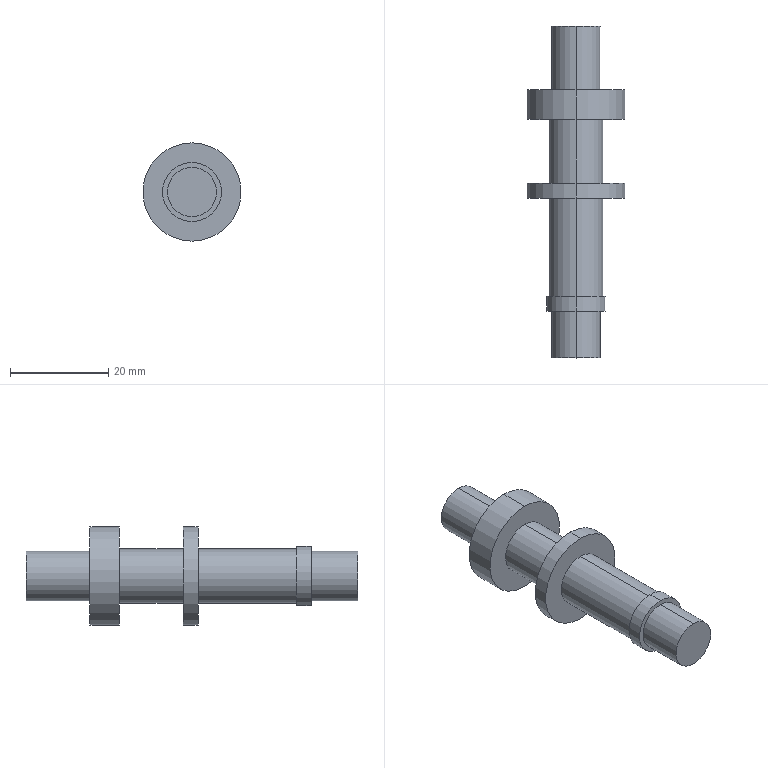Part | SolidWorks | features Revolution 1 | 1 solid | 22 faces | box 20 x 67.5 x 20 mm | volume 8070 mm3 | cylinder 14 | plane 8 | commonest cylinder face diameters 10 x4 11 x4 20 x4 12 x2
STEP:
#1=CARTESIAN_POINT('',(0.,67.5,-5.));
#2=VERTEX_POINT('',#1);
#3=CARTESIAN_POINT('',(0.,67.5,5.));
#4=VERTEX_POINT('',#3);
#5=CARTESIAN_POINT('',(0.,67.5,0.));
#6=DIRECTION('',(0.,-1.,0.));
#7=DIRECTION('',(0.,0.,-1.));
#8=AXIS2_PLACEMENT_3D('',#5,#6,#7);
#9=CIRCLE('',#8,5.);
#10=EDGE_CURVE('',#2,#4,#9,.T.);
#11=ORIENTED_EDGE('',*,*,#10,.T.);
#12=CARTESIAN_POINT('',(0.,54.5,5.));
#13=VERTEX_POINT('',#12);
#14=CARTESIAN_POINT('',(0.,-28.718,5.));
#15=DIRECTION('',(0.,-1.,0.));
#16=VECTOR('',#15,1000.);
#17=LINE('',#14,#16);
#18=EDGE_CURVE('',#4,#13,#17,.T.);
#19=ORIENTED_EDGE('',*,*,#18,.T.);
#20=CARTESIAN_POINT('',(0.,54.5,-5.));
#21=VERTEX_POINT('',#20);
#22=CARTESIAN_POINT('',(0.,54.5,0.));
#23=DIRECTION('',(0.,-1.,0.));
#24=DIRECTION('',(0.,0.,-1.));
#25=AXIS2_PLACEMENT_3D('',#22,#23,#24);
#26=CIRCLE('',#25,5.);
#27=EDGE_CURVE('',#21,#13,#26,.T.);
#28=ORIENTED_EDGE('',*,*,#27,.F.);
#29=CARTESIAN_POINT('',(0.,-28.718,-5.));
#30=DIRECTION('',(0.,-1.,0.));
#31=VECTOR('',#30,1000.);
#32=LINE('',#29,#31);
#33=EDGE_CURVE('',#2,#21,#32,.T.);
#34=ORIENTED_EDGE('',*,*,#33,.F.);
#35=EDGE_LOOP('',(#11,#19,#28,#34));
#36=FACE_OUTER_BOUND('',#35,.T.);
#37=CARTESIAN_POINT('',(0.,-28.718,0.));
#38=DIRECTION('',(0.,-1.,0.));
#39=DIRECTION('',(0.,0.,-1.));
#40=AXIS2_PLACEMENT_3D('',#37,#38,#39);
#41=CYLINDRICAL_SURFACE('',#40,5.);
#42=ADVANCED_FACE('',(#36),#41,.T.);
#43=CARTESIAN_POINT('',(0.,54.5,-10.));
#44=VERTEX_POINT('',#43);
#45=CARTESIAN_POINT('',(0.,54.5,10.));
#46=VERTEX_POINT('',#45);
#47=CARTESIAN_POINT('',(0.,54.5,0.));
#48=DIRECTION('',(0.,-1.,0.));
#49=DIRECTION('',(0.,0.,-1.));
#50=AXIS2_PLACEMENT_3D('',#47,#48,#49);
#51=CIRCLE('',#50,10.);
#52=EDGE_CURVE('',#44,#46,#51,.T.);
#53=ORIENTED_EDGE('',*,*,#52,.T.);
#54=CARTESIAN_POINT('',(0.,48.5,10.));
#55=VERTEX_POINT('',#54);
#56=CARTESIAN_POINT('',(0.,-28.718,10.));
#57=DIRECTION('',(0.,-1.,0.));
#58=VECTOR('',#57,1000.);
#59=LINE('',#56,#58);
#60=EDGE_CURVE('',#46,#55,#59,.T.);
#61=ORIENTED_EDGE('',*,*,#60,.T.);
#62=CARTESIAN_POINT('',(0.,48.5,-10.));
#63=VERTEX_POINT('',#62);
#64=CARTESIAN_POINT('',(0.,48.5,0.));
#65=DIRECTION('',(0.,-1.,0.));
#66=DIRECTION('',(0.,0.,-1.));
#67=AXIS2_PLACEMENT_3D('',#64,#65,#66);
#68=CIRCLE('',#67,10.);
#69=EDGE_CURVE('',#63,#55,#68,.T.);
#70=ORIENTED_EDGE('',*,*,#69,.F.);
#71=CARTESIAN_POINT('',(0.,-28.718,-10.));
#72=DIRECTION('',(0.,-1.,0.));
#73=VECTOR('',#72,1000.);
#74=LINE('',#71,#73);
#75=EDGE_CURVE('',#44,#63,#74,.T.);
#76=ORIENTED_EDGE('',*,*,#75,.F.);
#77=EDGE_LOOP('',(#53,#61,#70,#76));
#78=FACE_OUTER_BOUND('',#77,.T.);
#79=CARTESIAN_POINT('',(0.,-28.718,0.));
#80=DIRECTION('',(0.,-1.,0.));
#81=DIRECTION('',(0.,0.,-1.));
#82=AXIS2_PLACEMENT_3D('',#79,#80,#81);
#83=CYLINDRICAL_SURFACE('',#82,10.);
#84=ADVANCED_FACE('',(#78),#83,.T.);
#85=CARTESIAN_POINT('',(0.,48.5,-5.5));
#86=VERTEX_POINT('',#85);
#87=CARTESIAN_POINT('',(0.,48.5,5.5));
#88=VERTEX_POINT('',#87);
#89=CARTESIAN_POINT('',(0.,48.5,0.));
#90=DIRECTION('',(0.,-1.,0.));
#91=DIRECTION('',(0.,0.,-1.));
#92=AXIS2_PLACEMENT_3D('',#89,#90,#91);
#93=CIRCLE('',#92,5.5);
#94=EDGE_CURVE('',#86,#88,#93,.T.);
#95=ORIENTED_EDGE('',*,*,#94,.T.);
#96=CARTESIAN_POINT('',(0.,35.5,5.5));
#97=VERTEX_POINT('',#96);
#98=CARTESIAN_POINT('',(0.,-28.718,5.5));
#99=DIRECTION('',(0.,-1.,0.));
#100=VECTOR('',#99,1000.);
#101=LINE('',#98,#100);
#102=EDGE_CURVE('',#88,#97,#101,.T.);
#103=ORIENTED_EDGE('',*,*,#102,.T.);
#104=CARTESIAN_POINT('',(0.,35.5,-5.5));
#105=VERTEX_POINT('',#104);
#106=CARTESIAN_POINT('',(0.,35.5,0.));
#107=DIRECTION('',(0.,-1.,0.));
#108=DIRECTION('',(0.,0.,-1.));
#109=AXIS2_PLACEMENT_3D('',#106,#107,#108);
#110=CIRCLE('',#109,5.5);
#111=EDGE_CURVE('',#105,#97,#110,.T.);
#112=ORIENTED_EDGE('',*,*,#111,.F.);
#113=CARTESIAN_POINT('',(0.,-28.718,-5.5));
#114=DIRECTION('',(0.,-1.,0.));
#115=VECTOR('',#114,1000.);
#116=LINE('',#113,#115);
#117=EDGE_CURVE('',#86,#105,#116,.T.);
#118=ORIENTED_EDGE('',*,*,#117,.F.);
#119=EDGE_LOOP('',(#95,#103,#112,#118));
#120=FACE_OUTER_BOUND('',#119,.T.);
#121=CARTESIAN_POINT('',(0.,-28.718,0.));
#122=DIRECTION('',(0.,-1.,0.));
#123=DIRECTION('',(0.,0.,-1.));
#124=AXIS2_PLACEMENT_3D('',#121,#122,#123);
#125=CYLINDRICAL_SURFACE('',#124,5.5);
#126=ADVANCED_FACE('',(#120),#125,.T.);
#127=CARTESIAN_POINT('',(0.,35.5,-10.));
#128=VERTEX_POINT('',#127);
#129=CARTESIAN_POINT('',(0.,35.5,10.));
#130=VERTEX_POINT('',#129);
#131=CARTESIAN_POINT('',(0.,35.5,0.));
#132=DIRECTION('',(0.,-1.,0.));
#133=DIRECTION('',(0.,0.,-1.));
#134=AXIS2_PLACEMENT_3D('',#131,#132,#133);
#135=CIRCLE('',#134,10.);
#136=EDGE_CURVE('',#128,#130,#135,.T.);
#137=ORIENTED_EDGE('',*,*,#136,.T.);
#138=CARTESIAN_POINT('',(0.,32.5,10.));
#139=VERTEX_POINT('',#138);
#140=CARTESIAN_POINT('',(0.,-28.718,10.));
#141=DIRECTION('',(0.,-1.,0.));
#142=VECTOR('',#141,1000.);
#143=LINE('',#140,#142);
#144=EDGE_CURVE('',#130,#139,#143,.T.);
#145=ORIENTED_EDGE('',*,*,#144,.T.);
#146=CARTESIAN_POINT('',(0.,32.5,-10.));
#147=VERTEX_POINT('',#146);
#148=CARTESIAN_POINT('',(0.,32.5,0.));
#149=DIRECTION('',(0.,-1.,0.));
#150=DIRECTION('',(0.,0.,-1.));
#151=AXIS2_PLACEMENT_3D('',#148,#149,#150);
#152=CIRCLE('',#151,10.);
#153=EDGE_CURVE('',#147,#139,#152,.T.);
#154=ORIENTED_EDGE('',*,*,#153,.F.);
#155=CARTESIAN_POINT('',(0.,-28.718,-10.));
#156=DIRECTION('',(0.,-1.,0.));
#157=VECTOR('',#156,1000.);
#158=LINE('',#155,#157);
#159=EDGE_CURVE('',#128,#147,#158,.T.);
#160=ORIENTED_EDGE('',*,*,#159,.F.);
#161=EDGE_LOOP('',(#137,#145,#154,#160));
#162=FACE_OUTER_BOUND('',#161,.T.);
#163=CARTESIAN_POINT('',(0.,-28.718,0.));
#164=DIRECTION('',(0.,-1.,0.));
#165=DIRECTION('',(0.,0.,-1.));
#166=AXIS2_PLACEMENT_3D('',#163,#164,#165);
#167=CYLINDRICAL_SURFACE('',#166,10.);
#168=ADVANCED_FACE('',(#162),#167,.T.);
#169=CARTESIAN_POINT('',(0.,32.5,-5.5));
#170=VERTEX_POINT('',#169);
#171=CARTESIAN_POINT('',(0.,32.5,5.5));
#172=VERTEX_POINT('',#171);
#173=CARTESIAN_POINT('',(0.,32.5,0.));
#174=DIRECTION('',(0.,-1.,0.));
#175=DIRECTION('',(0.,0.,-1.));
#176=AXIS2_PLACEMENT_3D('',#173,#174,#175);
#177=CIRCLE('',#176,5.5);
#178=EDGE_CURVE('',#170,#172,#177,.T.);
#179=ORIENTED_EDGE('',*,*,#178,.T.);
#180=CARTESIAN_POINT('',(0.,12.5,5.5));
#181=VERTEX_POINT('',#180);
#182=CARTESIAN_POINT('',(0.,-28.718,5.5));
#183=DIRECTION('',(0.,-1.,0.));
#184=VECTOR('',#183,1000.);
#185=LINE('',#182,#184);
#186=EDGE_CURVE('',#172,#181,#185,.T.);
#187=ORIENTED_EDGE('',*,*,#186,.T.);
#188=CARTESIAN_POINT('',(0.,12.5,-5.5));
#189=VERTEX_POINT('',#188);
#190=CARTESIAN_POINT('',(0.,12.5,0.));
#191=DIRECTION('',(0.,-1.,0.));
#192=DIRECTION('',(0.,0.,-1.));
#193=AXIS2_PLACEMENT_3D('',#190,#191,#192);
#194=CIRCLE('',#193,5.5);
#195=EDGE_CURVE('',#189,#181,#194,.T.);
#196=ORIENTED_EDGE('',*,*,#195,.F.);
#197=CARTESIAN_POINT('',(0.,-28.718,-5.5));
#198=DIRECTION('',(0.,-1.,0.));
#199=VECTOR('',#198,1000.);
#200=LINE('',#197,#199);
#201=EDGE_CURVE('',#170,#189,#200,.T.);
#202=ORIENTED_EDGE('',*,*,#201,.F.);
#203=EDGE_LOOP('',(#179,#187,#196,#202));
#204=FACE_OUTER_BOUND('',#203,.T.);
#205=CARTESIAN_POINT('',(0.,-28.718,0.));
#206=DIRECTION('',(0.,-1.,0.));
#207=DIRECTION('',(0.,0.,-1.));
#208=AXIS2_PLACEMENT_3D('',#205,#206,#207);
#209=CYLINDRICAL_SURFACE('',#208,5.5);
#210=ADVANCED_FACE('',(#204),#209,.T.);
#211=CARTESIAN_POINT('',(0.,12.5,-6.));
#212=VERTEX_POINT('',#211);
#213=CARTESIAN_POINT('',(0.,12.5,6.));
#214=VERTEX_POINT('',#213);
#215=CARTESIAN_POINT('',(0.,12.5,0.));
#216=DIRECTION('',(0.,-1.,0.));
#217=DIRECTION('',(0.,0.,-1.));
#218=AXIS2_PLACEMENT_3D('',#215,#216,#217);
#219=CIRCLE('',#218,6.);
#220=EDGE_CURVE('',#212,#214,#219,.T.);
#221=ORIENTED_EDGE('',*,*,#220,.T.);
#222=CARTESIAN_POINT('',(0.,9.5,6.));
#223=VERTEX_POINT('',#222);
#224=CARTESIAN_POINT('',(0.,-28.718,6.));
#225=DIRECTION('',(0.,-1.,0.));
#226=VECTOR('',#225,1000.);
#227=LINE('',#224,#226);
#228=EDGE_CURVE('',#214,#223,#227,.T.);
#229=ORIENTED_EDGE('',*,*,#228,.T.);
#230=CARTESIAN_POINT('',(0.,9.5,-6.));
#231=VERTEX_POINT('',#230);
#232=CARTESIAN_POINT('',(0.,9.5,0.));
#233=DIRECTION('',(0.,-1.,0.));
#234=DIRECTION('',(0.,0.,-1.));
#235=AXIS2_PLACEMENT_3D('',#232,#233,#234);
#236=CIRCLE('',#235,6.);
#237=EDGE_CURVE('',#231,#223,#236,.T.);
#238=ORIENTED_EDGE('',*,*,#237,.F.);
#239=CARTESIAN_POINT('',(0.,-28.718,-6.));
#240=DIRECTION('',(0.,-1.,0.));
#241=VECTOR('',#240,1000.);
#242=LINE('',#239,#241);
#243=EDGE_CURVE('',#212,#231,#242,.T.);
#244=ORIENTED_EDGE('',*,*,#243,.F.);
#245=EDGE_LOOP('',(#221,#229,#238,#244));
#246=FACE_OUTER_BOUND('',#245,.T.);
#247=CARTESIAN_POINT('',(0.,-28.718,0.));
#248=DIRECTION('',(0.,-1.,0.));
#249=DIRECTION('',(0.,0.,-1.));
#250=AXIS2_PLACEMENT_3D('',#247,#248,#249);
#251=CYLINDRICAL_SURFACE('',#250,6.);
#252=ADVANCED_FACE('',(#246),#251,.T.);
#253=CARTESIAN_POINT('',(0.,9.5,-5.));
#254=VERTEX_POINT('',#253);
#255=CARTESIAN_POINT('',(0.,9.5,5.));
#256=VERTEX_POINT('',#255);
#257=CARTESIAN_POINT('',(0.,9.5,0.));
#258=DIRECTION('',(0.,-1.,0.));
#259=DIRECTION('',(0.,0.,-1.));
#260=AXIS2_PLACEMENT_3D('',#257,#258,#259);
#261=CIRCLE('',#260,5.);
#262=EDGE_CURVE('',#254,#256,#261,.T.);
#263=ORIENTED_EDGE('',*,*,#262,.T.);
#264=CARTESIAN_POINT('',(0.,0.,5.));
#265=VERTEX_POINT('',#264);
#266=CARTESIAN_POINT('',(0.,-28.718,5.));
#267=DIRECTION('',(0.,-1.,0.));
#268=VECTOR('',#267,1000.);
#269=LINE('',#266,#268);
#270=EDGE_CURVE('',#256,#265,#269,.T.);
#271=ORIENTED_EDGE('',*,*,#270,.T.);
#272=CARTESIAN_POINT('',(0.,0.,-5.));
#273=VERTEX_POINT('',#272);
#274=CARTESIAN_POINT('',(0.,0.,0.));
#275=DIRECTION('',(0.,-1.,0.));
#276=DIRECTION('',(0.,0.,-1.));
#277=AXIS2_PLACEMENT_3D('',#274,#275,#276);
#278=CIRCLE('',#277,5.);
#279=EDGE_CURVE('',#273,#265,#278,.T.);
#280=ORIENTED_EDGE('',*,*,#279,.F.);
#281=CARTESIAN_POINT('',(0.,-28.718,-5.));
#282=DIRECTION('',(0.,-1.,0.));
#283=VECTOR('',#282,1000.);
#284=LINE('',#281,#283);
#285=EDGE_CURVE('',#254,#273,#284,.T.);
#286=ORIENTED_EDGE('',*,*,#285,.F.);
#287=EDGE_LOOP('',(#263,#271,#280,#286));
#288=FACE_OUTER_BOUND('',#287,.T.);
#289=CARTESIAN_POINT('',(0.,-28.718,0.));
#290=DIRECTION('',(0.,-1.,0.));
#291=DIRECTION('',(0.,0.,-1.));
#292=AXIS2_PLACEMENT_3D('',#289,#290,#291);
#293=CYLINDRICAL_SURFACE('',#292,5.);
#294=ADVANCED_FACE('',(#288),#293,.T.);
#295=ORIENTED_EDGE('',*,*,#279,.T.);
#296=CARTESIAN_POINT('',(0.,0.,0.));
#297=DIRECTION('',(0.,-1.,0.));
#298=DIRECTION('',(0.,0.,-1.));
#299=AXIS2_PLACEMENT_3D('',#296,#297,#298);
#300=CIRCLE('',#299,5.);
#301=EDGE_CURVE('',#265,#273,#300,.T.);
#302=ORIENTED_EDGE('',*,*,#301,.T.);
#303=EDGE_LOOP('',(#295,#302));
#304=FACE_OUTER_BOUND('',#303,.T.);
#305=CARTESIAN_POINT('',(0.,0.,0.));
#306=DIRECTION('',(0.,-1.,0.));
#307=DIRECTION('',(0.,0.,-1.));
#308=AXIS2_PLACEMENT_3D('',#305,#306,#307);
#309=PLANE('',#308);
#310=ADVANCED_FACE('',(#304),#309,.T.);
#311=ORIENTED_EDGE('',*,*,#270,.F.);
#312=CARTESIAN_POINT('',(0.,9.5,0.));
#313=DIRECTION('',(0.,-1.,0.));
#314=DIRECTION('',(0.,0.,-1.));
#315=AXIS2_PLACEMENT_3D('',#312,#313,#314);
#316=CIRCLE('',#315,5.);
#317=EDGE_CURVE('',#256,#254,#316,.T.);
#318=ORIENTED_EDGE('',*,*,#317,.T.);
#319=ORIENTED_EDGE('',*,*,#285,.T.);
#320=ORIENTED_EDGE('',*,*,#301,.F.);
#321=EDGE_LOOP('',(#311,#318,#319,#320));
#322=FACE_OUTER_BOUND('',#321,.T.);
#323=CARTESIAN_POINT('',(0.,-28.718,0.));
#324=DIRECTION('',(0.,-1.,0.));
#325=DIRECTION('',(0.,0.,-1.));
#326=AXIS2_PLACEMENT_3D('',#323,#324,#325);
#327=CYLINDRICAL_SURFACE('',#326,5.);
#328=ADVANCED_FACE('',(#322),#327,.T.);
#329=ORIENTED_EDGE('',*,*,#237,.T.);
#330=CARTESIAN_POINT('',(0.,9.5,0.));
#331=DIRECTION('',(0.,-1.,0.));
#332=DIRECTION('',(0.,0.,-1.));
#333=AXIS2_PLACEMENT_3D('',#330,#331,#332);
#334=CIRCLE('',#333,6.);
#335=EDGE_CURVE('',#223,#231,#334,.T.);
#336=ORIENTED_EDGE('',*,*,#335,.T.);
#337=EDGE_LOOP('',(#329,#336));
#338=FACE_OUTER_BOUND('',#337,.T.);
#339=ORIENTED_EDGE('',*,*,#262,.F.);
#340=ORIENTED_EDGE('',*,*,#317,.F.);
#341=EDGE_LOOP('',(#339,#340));
#342=FACE_BOUND('',#341,.T.);
#343=CARTESIAN_POINT('',(5.,9.5,0.));
#344=DIRECTION('',(0.,-1.,0.));
#345=DIRECTION('',(0.,0.,-1.));
#346=AXIS2_PLACEMENT_3D('',#343,#344,#345);
#347=PLANE('',#346);
#348=ADVANCED_FACE('',(#338,#342),#347,.T.);
#349=ORIENTED_EDGE('',*,*,#228,.F.);
#350=CARTESIAN_POINT('',(0.,12.5,0.));
#351=DIRECTION('',(0.,-1.,0.));
#352=DIRECTION('',(0.,0.,-1.));
#353=AXIS2_PLACEMENT_3D('',#350,#351,#352);
#354=CIRCLE('',#353,6.);
#355=EDGE_CURVE('',#214,#212,#354,.T.);
#356=ORIENTED_EDGE('',*,*,#355,.T.);
#357=ORIENTED_EDGE('',*,*,#243,.T.);
#358=ORIENTED_EDGE('',*,*,#335,.F.);
#359=EDGE_LOOP('',(#349,#356,#357,#358));
#360=FACE_OUTER_BOUND('',#359,.T.);
#361=CARTESIAN_POINT('',(0.,-28.718,0.));
#362=DIRECTION('',(0.,-1.,0.));
#363=DIRECTION('',(0.,0.,-1.));
#364=AXIS2_PLACEMENT_3D('',#361,#362,#363);
#365=CYLINDRICAL_SURFACE('',#364,6.);
#366=ADVANCED_FACE('',(#360),#365,.T.);
#367=ORIENTED_EDGE('',*,*,#195,.T.);
#368=CARTESIAN_POINT('',(0.,12.5,0.));
#369=DIRECTION('',(0.,-1.,0.));
#370=DIRECTION('',(0.,0.,-1.));
#371=AXIS2_PLACEMENT_3D('',#368,#369,#370);
#372=CIRCLE('',#371,5.5);
#373=EDGE_CURVE('',#181,#189,#372,.T.);
#374=ORIENTED_EDGE('',*,*,#373,.T.);
#375=EDGE_LOOP('',(#367,#374));
#376=FACE_BOUND('',#375,.T.);
#377=ORIENTED_EDGE('',*,*,#220,.F.);
#378=ORIENTED_EDGE('',*,*,#355,.F.);
#379=EDGE_LOOP('',(#377,#378));
#380=FACE_OUTER_BOUND('',#379,.T.);
#381=CARTESIAN_POINT('',(6.,12.5,0.));
#382=DIRECTION('',(0.,1.,0.));
#383=DIRECTION('',(0.,0.,1.));
#384=AXIS2_PLACEMENT_3D('',#381,#382,#383);
#385=PLANE('',#384);
#386=ADVANCED_FACE('',(#376,#380),#385,.T.);
#387=ORIENTED_EDGE('',*,*,#186,.F.);
#388=CARTESIAN_POINT('',(0.,32.5,0.));
#389=DIRECTION('',(0.,-1.,0.));
#390=DIRECTION('',(0.,0.,-1.));
#391=AXIS2_PLACEMENT_3D('',#388,#389,#390);
#392=CIRCLE('',#391,5.5);
#393=EDGE_CURVE('',#172,#170,#392,.T.);
#394=ORIENTED_EDGE('',*,*,#393,.T.);
#395=ORIENTED_EDGE('',*,*,#201,.T.);
#396=ORIENTED_EDGE('',*,*,#373,.F.);
#397=EDGE_LOOP('',(#387,#394,#395,#396));
#398=FACE_OUTER_BOUND('',#397,.T.);
#399=CARTESIAN_POINT('',(0.,-28.718,0.));
#400=DIRECTION('',(0.,-1.,0.));
#401=DIRECTION('',(0.,0.,-1.));
#402=AXIS2_PLACEMENT_3D('',#399,#400,#401);
#403=CYLINDRICAL_SURFACE('',#402,5.5);
#404=ADVANCED_FACE('',(#398),#403,.T.);
#405=ORIENTED_EDGE('',*,*,#153,.T.);
#406=CARTESIAN_POINT('',(0.,32.5,0.));
#407=DIRECTION('',(0.,-1.,0.));
#408=DIRECTION('',(0.,0.,-1.));
#409=AXIS2_PLACEMENT_3D('',#406,#407,#408);
#410=CIRCLE('',#409,10.);
#411=EDGE_CURVE('',#139,#147,#410,.T.);
#412=ORIENTED_EDGE('',*,*,#411,.T.);
#413=EDGE_LOOP('',(#405,#412));
#414=FACE_OUTER_BOUND('',#413,.T.);
#415=ORIENTED_EDGE('',*,*,#178,.F.);
#416=ORIENTED_EDGE('',*,*,#393,.F.);
#417=EDGE_LOOP('',(#415,#416));
#418=FACE_BOUND('',#417,.T.);
#419=CARTESIAN_POINT('',(5.5,32.5,0.));
#420=DIRECTION('',(0.,-1.,0.));
#421=DIRECTION('',(0.,0.,-1.));
#422=AXIS2_PLACEMENT_3D('',#419,#420,#421);
#423=PLANE('',#422);
#424=ADVANCED_FACE('',(#414,#418),#423,.T.);
#425=ORIENTED_EDGE('',*,*,#144,.F.);
#426=CARTESIAN_POINT('',(0.,35.5,0.));
#427=DIRECTION('',(0.,-1.,0.));
#428=DIRECTION('',(0.,0.,-1.));
#429=AXIS2_PLACEMENT_3D('',#426,#427,#428);
#430=CIRCLE('',#429,10.);
#431=EDGE_CURVE('',#130,#128,#430,.T.);
#432=ORIENTED_EDGE('',*,*,#431,.T.);
#433=ORIENTED_EDGE('',*,*,#159,.T.);
#434=ORIENTED_EDGE('',*,*,#411,.F.);
#435=EDGE_LOOP('',(#425,#432,#433,#434));
#436=FACE_OUTER_BOUND('',#435,.T.);
#437=CARTESIAN_POINT('',(0.,-28.718,0.));
#438=DIRECTION('',(0.,-1.,0.));
#439=DIRECTION('',(0.,0.,-1.));
#440=AXIS2_PLACEMENT_3D('',#437,#438,#439);
#441=CYLINDRICAL_SURFACE('',#440,10.);
#442=ADVANCED_FACE('',(#436),#441,.T.);
#443=ORIENTED_EDGE('',*,*,#111,.T.);
#444=CARTESIAN_POINT('',(0.,35.5,0.));
#445=DIRECTION('',(0.,-1.,0.));
#446=DIRECTION('',(0.,0.,-1.));
#447=AXIS2_PLACEMENT_3D('',#444,#445,#446);
#448=CIRCLE('',#447,5.5);
#449=EDGE_CURVE('',#97,#105,#448,.T.);
#450=ORIENTED_EDGE('',*,*,#449,.T.);
#451=EDGE_LOOP('',(#443,#450));
#452=FACE_BOUND('',#451,.T.);
#453=ORIENTED_EDGE('',*,*,#136,.F.);
#454=ORIENTED_EDGE('',*,*,#431,.F.);
#455=EDGE_LOOP('',(#453,#454));
#456=FACE_OUTER_BOUND('',#455,.T.);
#457=CARTESIAN_POINT('',(10.,35.5,0.));
#458=DIRECTION('',(0.,1.,0.));
#459=DIRECTION('',(0.,0.,1.));
#460=AXIS2_PLACEMENT_3D('',#457,#458,#459);
#461=PLANE('',#460);
#462=ADVANCED_FACE('',(#452,#456),#461,.T.);
#463=ORIENTED_EDGE('',*,*,#102,.F.);
#464=CARTESIAN_POINT('',(0.,48.5,0.));
#465=DIRECTION('',(0.,-1.,0.));
#466=DIRECTION('',(0.,0.,-1.));
#467=AXIS2_PLACEMENT_3D('',#464,#465,#466);
#468=CIRCLE('',#467,5.5);
#469=EDGE_CURVE('',#88,#86,#468,.T.);
#470=ORIENTED_EDGE('',*,*,#469,.T.);
#471=ORIENTED_EDGE('',*,*,#117,.T.);
#472=ORIENTED_EDGE('',*,*,#449,.F.);
#473=EDGE_LOOP('',(#463,#470,#471,#472));
#474=FACE_OUTER_BOUND('',#473,.T.);
#475=CARTESIAN_POINT('',(0.,-28.718,0.));
#476=DIRECTION('',(0.,-1.,0.));
#477=DIRECTION('',(0.,0.,-1.));
#478=AXIS2_PLACEMENT_3D('',#475,#476,#477);
#479=CYLINDRICAL_SURFACE('',#478,5.5);
#480=ADVANCED_FACE('',(#474),#479,.T.);
#481=ORIENTED_EDGE('',*,*,#69,.T.);
#482=CARTESIAN_POINT('',(0.,48.5,0.));
#483=DIRECTION('',(0.,-1.,0.));
#484=DIRECTION('',(0.,0.,-1.));
#485=AXIS2_PLACEMENT_3D('',#482,#483,#484);
#486=CIRCLE('',#485,10.);
#487=EDGE_CURVE('',#55,#63,#486,.T.);
#488=ORIENTED_EDGE('',*,*,#487,.T.);
#489=EDGE_LOOP('',(#481,#488));
#490=FACE_OUTER_BOUND('',#489,.T.);
#491=ORIENTED_EDGE('',*,*,#94,.F.);
#492=ORIENTED_EDGE('',*,*,#469,.F.);
#493=EDGE_LOOP('',(#491,#492));
#494=FACE_BOUND('',#493,.T.);
#495=CARTESIAN_POINT('',(5.5,48.5,0.));
#496=DIRECTION('',(0.,-1.,0.));
#497=DIRECTION('',(0.,0.,-1.));
#498=AXIS2_PLACEMENT_3D('',#495,#496,#497);
#499=PLANE('',#498);
#500=ADVANCED_FACE('',(#490,#494),#499,.T.);
#501=ORIENTED_EDGE('',*,*,#60,.F.);
#502=CARTESIAN_POINT('',(0.,54.5,0.));
#503=DIRECTION('',(0.,-1.,0.));
#504=DIRECTION('',(0.,0.,-1.));
#505=AXIS2_PLACEMENT_3D('',#502,#503,#504);
#506=CIRCLE('',#505,10.);
#507=EDGE_CURVE('',#46,#44,#506,.T.);
#508=ORIENTED_EDGE('',*,*,#507,.T.);
#509=ORIENTED_EDGE('',*,*,#75,.T.);
#510=ORIENTED_EDGE('',*,*,#487,.F.);
#511=EDGE_LOOP('',(#501,#508,#509,#510));
#512=FACE_OUTER_BOUND('',#511,.T.);
#513=CARTESIAN_POINT('',(0.,-28.718,0.));
#514=DIRECTION('',(0.,-1.,0.));
#515=DIRECTION('',(0.,0.,-1.));
#516=AXIS2_PLACEMENT_3D('',#513,#514,#515);
#517=CYLINDRICAL_SURFACE('',#516,10.);
#518=ADVANCED_FACE('',(#512),#517,.T.);
#519=ORIENTED_EDGE('',*,*,#27,.T.);
#520=CARTESIAN_POINT('',(0.,54.5,0.));
#521=DIRECTION('',(0.,-1.,0.));
#522=DIRECTION('',(0.,0.,-1.));
#523=AXIS2_PLACEMENT_3D('',#520,#521,#522);
#524=CIRCLE('',#523,5.);
#525=EDGE_CURVE('',#13,#21,#524,.T.);
#526=ORIENTED_EDGE('',*,*,#525,.T.);
#527=EDGE_LOOP('',(#519,#526));
#528=FACE_BOUND('',#527,.T.);
#529=ORIENTED_EDGE('',*,*,#52,.F.);
#530=ORIENTED_EDGE('',*,*,#507,.F.);
#531=EDGE_LOOP('',(#529,#530));
#532=FACE_OUTER_BOUND('',#531,.T.);
#533=CARTESIAN_POINT('',(10.,54.5,0.));
#534=DIRECTION('',(0.,1.,0.));
#535=DIRECTION('',(0.,0.,1.));
#536=AXIS2_PLACEMENT_3D('',#533,#534,#535);
#537=PLANE('',#536);
#538=ADVANCED_FACE('',(#528,#532),#537,.T.);
#539=ORIENTED_EDGE('',*,*,#18,.F.);
#540=CARTESIAN_POINT('',(0.,67.5,0.));
#541=DIRECTION('',(0.,-1.,0.));
#542=DIRECTION('',(0.,0.,-1.));
#543=AXIS2_PLACEMENT_3D('',#540,#541,#542);
#544=CIRCLE('',#543,5.);
#545=EDGE_CURVE('',#4,#2,#544,.T.);
#546=ORIENTED_EDGE('',*,*,#545,.T.);
#547=ORIENTED_EDGE('',*,*,#33,.T.);
#548=ORIENTED_EDGE('',*,*,#525,.F.);
#549=EDGE_LOOP('',(#539,#546,#547,#548));
#550=FACE_OUTER_BOUND('',#549,.T.);
#551=CARTESIAN_POINT('',(0.,-28.718,0.));
#552=DIRECTION('',(0.,-1.,0.));
#553=DIRECTION('',(0.,0.,-1.));
#554=AXIS2_PLACEMENT_3D('',#551,#552,#553);
#555=CYLINDRICAL_SURFACE('',#554,5.);
#556=ADVANCED_FACE('',(#550),#555,.T.);
#557=ORIENTED_EDGE('',*,*,#10,.F.);
#558=ORIENTED_EDGE('',*,*,#545,.F.);
#559=EDGE_LOOP('',(#557,#558));
#560=FACE_OUTER_BOUND('',#559,.T.);
#561=CARTESIAN_POINT('',(5.,67.5,0.));
#562=DIRECTION('',(0.,1.,0.));
#563=DIRECTION('',(0.,0.,1.));
#564=AXIS2_PLACEMENT_3D('',#561,#562,#563);
#565=PLANE('',#564);
#566=ADVANCED_FACE('',(#560),#565,.T.);
#567=CLOSED_SHELL('',(#42,#84,#126,#168,#210,#252,#294,#310,#328,#348,#366,#386,#404,#424,#442,#462,#480,#500,#518,#538,#556,#566));
#568=MANIFOLD_SOLID_BREP('',#567);
#569=CARTESIAN_POINT('',(0.,0.,0.));
#570=DIRECTION('',(0.,0.,1.));
#571=DIRECTION('',(1.,0.,0.));
#572=AXIS2_PLACEMENT_3D('',#569,#570,#571);
#573=(LENGTH_UNIT()NAMED_UNIT(*)SI_UNIT(.MILLI.,.METRE.));
#574=UNCERTAINTY_MEASURE_WITH_UNIT(LENGTH_MEASURE(0.00001),#573,'','');
#575=(NAMED_UNIT(*)PLANE_ANGLE_UNIT()SI_UNIT($,.RADIAN.));
#576=(NAMED_UNIT(*)SI_UNIT($,.STERADIAN.)SOLID_ANGLE_UNIT());
#577=(GEOMETRIC_REPRESENTATION_CONTEXT(3)GLOBAL_UNCERTAINTY_ASSIGNED_CONTEXT((#574))GLOBAL_UNIT_ASSIGNED_CONTEXT((#573,#575,#576))REPRESENTATION_CONTEXT('',''));
#578=ADVANCED_BREP_SHAPE_REPRESENTATION('',(#568,#572),#577);